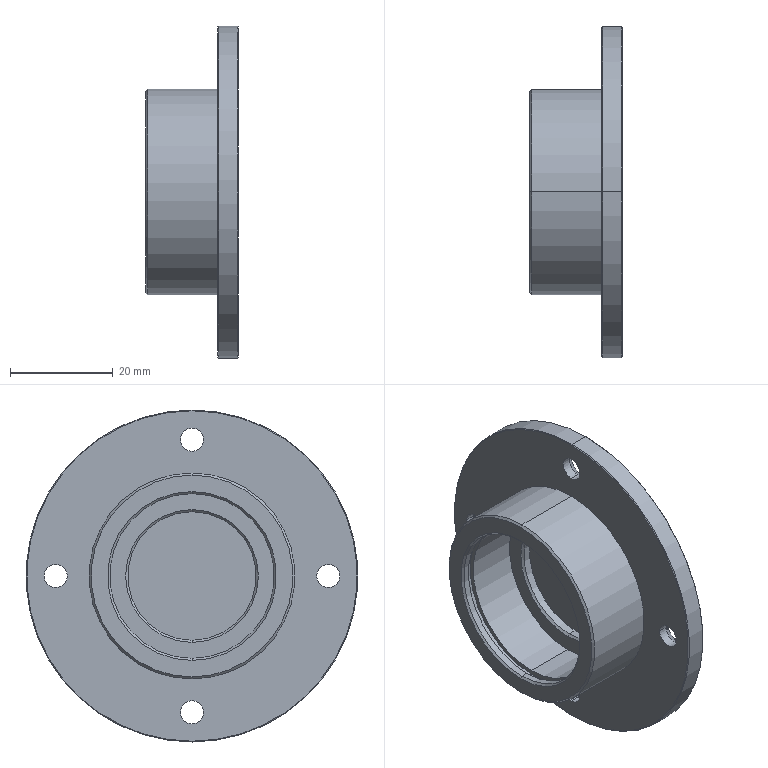Part | SolidWorks | features CirPattern 2, Chamfer 1, HoleWzd 1, ICE 1, RevCut 1, Revolution 1 | 1 solid | 45 faces | box 18 x 64.5 x 64.5 mm | volume 18637 mm3 | cylinder 20 | cone 18 | plane 7 | commonest cylinder face diameters 4.5 x8 32 x4 25 x2 33.7 x2 40 x2 64.5 x2
STEP:
#1=CARTESIAN_POINT('',(14.15,0.,32.25));
#2=VERTEX_POINT('',#1);
#3=CARTESIAN_POINT('',(14.15,0.,-32.25));
#4=VERTEX_POINT('',#3);
#5=CARTESIAN_POINT('',(14.15,0.,0.));
#6=DIRECTION('',(-1.,0.,0.));
#7=DIRECTION('',(0.,0.,-1.));
#8=AXIS2_PLACEMENT_3D('',#5,#6,#7);
#9=CIRCLE('',#8,32.25);
#10=EDGE_CURVE('',#2,#4,#9,.T.);
#11=ORIENTED_EDGE('',*,*,#10,.F.);
#12=CARTESIAN_POINT('',(17.85,0.,32.25));
#13=VERTEX_POINT('',#12);
#14=CARTESIAN_POINT('',(8.,0.,32.25));
#15=DIRECTION('',(1.,0.,0.));
#16=VECTOR('',#15,1000.);
#17=LINE('',#14,#16);
#18=EDGE_CURVE('',#2,#13,#17,.T.);
#19=ORIENTED_EDGE('',*,*,#18,.T.);
#20=CARTESIAN_POINT('',(17.85,0.,-32.25));
#21=VERTEX_POINT('',#20);
#22=CARTESIAN_POINT('',(17.85,0.,0.));
#23=DIRECTION('',(1.,0.,0.));
#24=DIRECTION('',(0.,0.,1.));
#25=AXIS2_PLACEMENT_3D('',#22,#23,#24);
#26=CIRCLE('',#25,32.25);
#27=EDGE_CURVE('',#21,#13,#26,.T.);
#28=ORIENTED_EDGE('',*,*,#27,.F.);
#29=CARTESIAN_POINT('',(8.,0.,-32.25));
#30=DIRECTION('',(1.,0.,0.));
#31=VECTOR('',#30,1000.);
#32=LINE('',#29,#31);
#33=EDGE_CURVE('',#4,#21,#32,.T.);
#34=ORIENTED_EDGE('',*,*,#33,.F.);
#35=EDGE_LOOP('',(#11,#19,#28,#34));
#36=FACE_OUTER_BOUND('',#35,.T.);
#37=CARTESIAN_POINT('',(8.,0.,0.));
#38=DIRECTION('',(1.,0.,0.));
#39=DIRECTION('',(0.,0.,-1.));
#40=AXIS2_PLACEMENT_3D('',#37,#38,#39);
#41=CYLINDRICAL_SURFACE('',#40,32.25);
#42=ADVANCED_FACE('',(#36),#41,.T.);
#43=CARTESIAN_POINT('',(0.,0.,19.6));
#44=VERTEX_POINT('',#43);
#45=CARTESIAN_POINT('',(0.,0.,-19.6));
#46=VERTEX_POINT('',#45);
#47=CARTESIAN_POINT('',(0.,0.,0.));
#48=DIRECTION('',(-1.,0.,0.));
#49=DIRECTION('',(0.,0.,-1.));
#50=AXIS2_PLACEMENT_3D('',#47,#48,#49);
#51=CIRCLE('',#50,19.6);
#52=EDGE_CURVE('',#44,#46,#51,.T.);
#53=ORIENTED_EDGE('',*,*,#52,.F.);
#54=CARTESIAN_POINT('',(0.4,0.,20.));
#55=VERTEX_POINT('',#54);
#56=CARTESIAN_POINT('',(0.,0.,19.6));
#57=DIRECTION('',(0.7071,0.,0.7071));
#58=VECTOR('',#57,1000.);
#59=LINE('',#56,#58);
#60=EDGE_CURVE('',#44,#55,#59,.T.);
#61=ORIENTED_EDGE('',*,*,#60,.T.);
#62=CARTESIAN_POINT('',(0.4,0.,-20.));
#63=VERTEX_POINT('',#62);
#64=CARTESIAN_POINT('',(0.4,0.,0.));
#65=DIRECTION('',(1.,0.,0.));
#66=DIRECTION('',(0.,0.,-1.));
#67=AXIS2_PLACEMENT_3D('',#64,#65,#66);
#68=CIRCLE('',#67,20.);
#69=EDGE_CURVE('',#63,#55,#68,.T.);
#70=ORIENTED_EDGE('',*,*,#69,.F.);
#71=CARTESIAN_POINT('',(0.,0.,-19.6));
#72=DIRECTION('',(0.7071,0.,-0.7071));
#73=VECTOR('',#72,1000.);
#74=LINE('',#71,#73);
#75=EDGE_CURVE('',#46,#63,#74,.T.);
#76=ORIENTED_EDGE('',*,*,#75,.F.);
#77=EDGE_LOOP('',(#53,#61,#70,#76));
#78=FACE_OUTER_BOUND('',#77,.T.);
#79=CARTESIAN_POINT('',(0.,0.,0.));
#80=DIRECTION('',(1.,0.,0.));
#81=DIRECTION('',(0.,0.,-1.));
#82=AXIS2_PLACEMENT_3D('',#79,#80,#81);
#83=CONICAL_SURFACE('',#82,19.6,0.7854);
#84=ADVANCED_FACE('',(#78),#83,.T.);
#85=CARTESIAN_POINT('',(0.4,0.,-16.));
#86=VERTEX_POINT('',#85);
#87=CARTESIAN_POINT('',(0.4,0.,16.));
#88=VERTEX_POINT('',#87);
#89=CARTESIAN_POINT('',(0.4,0.,0.));
#90=DIRECTION('',(-1.,0.,0.));
#91=DIRECTION('',(0.,0.,-1.));
#92=AXIS2_PLACEMENT_3D('',#89,#90,#91);
#93=CIRCLE('',#92,16.);
#94=EDGE_CURVE('',#86,#88,#93,.T.);
#95=ORIENTED_EDGE('',*,*,#94,.F.);
#96=CARTESIAN_POINT('',(0.,0.,-16.4));
#97=VERTEX_POINT('',#96);
#98=CARTESIAN_POINT('',(0.4,0.,-16.));
#99=DIRECTION('',(-0.7071,0.,-0.7071));
#100=VECTOR('',#99,1000.);
#101=LINE('',#98,#100);
#102=EDGE_CURVE('',#86,#97,#101,.T.);
#103=ORIENTED_EDGE('',*,*,#102,.T.);
#104=CARTESIAN_POINT('',(0.,0.,16.4));
#105=VERTEX_POINT('',#104);
#106=CARTESIAN_POINT('',(0.,0.,0.));
#107=DIRECTION('',(1.,0.,0.));
#108=DIRECTION('',(0.,0.,-1.));
#109=AXIS2_PLACEMENT_3D('',#106,#107,#108);
#110=CIRCLE('',#109,16.4);
#111=EDGE_CURVE('',#105,#97,#110,.T.);
#112=ORIENTED_EDGE('',*,*,#111,.F.);
#113=CARTESIAN_POINT('',(0.4,0.,16.));
#114=DIRECTION('',(-0.7071,0.,0.7071));
#115=VECTOR('',#114,1000.);
#116=LINE('',#113,#115);
#117=EDGE_CURVE('',#88,#105,#116,.T.);
#118=ORIENTED_EDGE('',*,*,#117,.F.);
#119=EDGE_LOOP('',(#95,#103,#112,#118));
#120=FACE_OUTER_BOUND('',#119,.T.);
#121=CARTESIAN_POINT('',(0.4,0.,0.));
#122=DIRECTION('',(-1.,0.,0.));
#123=DIRECTION('',(0.,0.,1.));
#124=AXIS2_PLACEMENT_3D('',#121,#122,#123);
#125=CONICAL_SURFACE('',#124,16.,0.7854);
#126=ADVANCED_FACE('',(#120),#125,.F.);
#127=CARTESIAN_POINT('',(13.4,0.,-12.5));
#128=VERTEX_POINT('',#127);
#129=CARTESIAN_POINT('',(13.4,0.,12.5));
#130=VERTEX_POINT('',#129);
#131=CARTESIAN_POINT('',(13.4,0.,0.));
#132=DIRECTION('',(-1.,0.,0.));
#133=DIRECTION('',(0.,0.,-1.));
#134=AXIS2_PLACEMENT_3D('',#131,#132,#133);
#135=CIRCLE('',#134,12.5);
#136=EDGE_CURVE('',#128,#130,#135,.T.);
#137=ORIENTED_EDGE('',*,*,#136,.F.);
#138=CARTESIAN_POINT('',(13.,0.,-12.9));
#139=VERTEX_POINT('',#138);
#140=CARTESIAN_POINT('',(13.4,0.,-12.5));
#141=DIRECTION('',(-0.7071,0.,-0.7071));
#142=VECTOR('',#141,1000.);
#143=LINE('',#140,#142);
#144=EDGE_CURVE('',#128,#139,#143,.T.);
#145=ORIENTED_EDGE('',*,*,#144,.T.);
#146=CARTESIAN_POINT('',(13.,0.,12.9));
#147=VERTEX_POINT('',#146);
#148=CARTESIAN_POINT('',(13.,0.,0.));
#149=DIRECTION('',(1.,0.,0.));
#150=DIRECTION('',(0.,0.,-1.));
#151=AXIS2_PLACEMENT_3D('',#148,#149,#150);
#152=CIRCLE('',#151,12.9);
#153=EDGE_CURVE('',#147,#139,#152,.T.);
#154=ORIENTED_EDGE('',*,*,#153,.F.);
#155=CARTESIAN_POINT('',(13.4,0.,12.5));
#156=DIRECTION('',(-0.7071,0.,0.7071));
#157=VECTOR('',#156,1000.);
#158=LINE('',#155,#157);
#159=EDGE_CURVE('',#130,#147,#158,.T.);
#160=ORIENTED_EDGE('',*,*,#159,.F.);
#161=EDGE_LOOP('',(#137,#145,#154,#160));
#162=FACE_OUTER_BOUND('',#161,.T.);
#163=CARTESIAN_POINT('',(13.4,0.,0.));
#164=DIRECTION('',(-1.,0.,0.));
#165=DIRECTION('',(0.,0.,1.));
#166=AXIS2_PLACEMENT_3D('',#163,#164,#165);
#167=CONICAL_SURFACE('',#166,12.5,0.7854);
#168=ADVANCED_FACE('',(#162),#167,.F.);
#169=CARTESIAN_POINT('',(15.75,28.75,0.));
#170=VERTEX_POINT('',#169);
#171=CARTESIAN_POINT('',(15.75,24.25,0.));
#172=VERTEX_POINT('',#171);
#173=CARTESIAN_POINT('',(15.75,26.5,0.));
#174=DIRECTION('',(-1.,0.,0.));
#175=DIRECTION('',(0.,-1.,0.));
#176=AXIS2_PLACEMENT_3D('',#173,#174,#175);
#177=CIRCLE('',#176,2.25);
#178=EDGE_CURVE('',#170,#172,#177,.T.);
#179=ORIENTED_EDGE('',*,*,#178,.F.);
#180=CARTESIAN_POINT('',(14.,28.75,0.));
#181=VERTEX_POINT('',#180);
#182=CARTESIAN_POINT('',(14.,28.75,0.));
#183=DIRECTION('',(-1.,0.,0.));
#184=VECTOR('',#183,1000.);
#185=LINE('',#182,#184);
#186=EDGE_CURVE('',#170,#181,#185,.T.);
#187=ORIENTED_EDGE('',*,*,#186,.T.);
#188=CARTESIAN_POINT('',(14.,24.25,0.));
#189=VERTEX_POINT('',#188);
#190=CARTESIAN_POINT('',(14.,26.5,0.));
#191=DIRECTION('',(-1.,0.,0.));
#192=DIRECTION('',(0.,-1.,0.));
#193=AXIS2_PLACEMENT_3D('',#190,#191,#192);
#194=CIRCLE('',#193,2.25);
#195=EDGE_CURVE('',#181,#189,#194,.T.);
#196=ORIENTED_EDGE('',*,*,#195,.T.);
#197=CARTESIAN_POINT('',(14.,24.25,0.));
#198=DIRECTION('',(-1.,0.,0.));
#199=VECTOR('',#198,1000.);
#200=LINE('',#197,#199);
#201=EDGE_CURVE('',#172,#189,#200,.T.);
#202=ORIENTED_EDGE('',*,*,#201,.F.);
#203=EDGE_LOOP('',(#179,#187,#196,#202));
#204=FACE_OUTER_BOUND('',#203,.T.);
#205=CARTESIAN_POINT('',(14.,26.5,0.));
#206=DIRECTION('',(-1.,0.,0.));
#207=DIRECTION('',(0.,-1.,0.));
#208=AXIS2_PLACEMENT_3D('',#205,#206,#207);
#209=CYLINDRICAL_SURFACE('',#208,2.25);
#210=ADVANCED_FACE('',(#204),#209,.F.);
#211=ORIENTED_EDGE('',*,*,#178,.T.);
#212=CARTESIAN_POINT('',(18.,22.,0.));
#213=VERTEX_POINT('',#212);
#214=CARTESIAN_POINT('',(18.,22.,0.));
#215=DIRECTION('',(0.7071,-0.7071,0.));
#216=VECTOR('',#215,1000.);
#217=LINE('',#214,#216);
#218=EDGE_CURVE('',#172,#213,#217,.T.);
#219=ORIENTED_EDGE('',*,*,#218,.T.);
#220=CARTESIAN_POINT('',(18.,31.,0.));
#221=VERTEX_POINT('',#220);
#222=CARTESIAN_POINT('',(18.,26.5,0.));
#223=DIRECTION('',(-1.,0.,0.));
#224=DIRECTION('',(0.,-1.,0.));
#225=AXIS2_PLACEMENT_3D('',#222,#223,#224);
#226=CIRCLE('',#225,4.5);
#227=EDGE_CURVE('',#221,#213,#226,.T.);
#228=ORIENTED_EDGE('',*,*,#227,.F.);
#229=CARTESIAN_POINT('',(18.,31.,0.));
#230=DIRECTION('',(0.7071,0.7071,0.));
#231=VECTOR('',#230,1000.);
#232=LINE('',#229,#231);
#233=EDGE_CURVE('',#170,#221,#232,.T.);
#234=ORIENTED_EDGE('',*,*,#233,.F.);
#235=EDGE_LOOP('',(#211,#219,#228,#234));
#236=FACE_OUTER_BOUND('',#235,.T.);
#237=CARTESIAN_POINT('',(18.,26.5,0.));
#238=DIRECTION('',(1.,0.,0.));
#239=DIRECTION('',(0.,1.,0.));
#240=AXIS2_PLACEMENT_3D('',#237,#238,#239);
#241=CONICAL_SURFACE('',#240,4.5,0.7854);
#242=ADVANCED_FACE('',(#236),#241,.F.);
#243=CARTESIAN_POINT('',(15.75,0.,28.75));
#244=VERTEX_POINT('',#243);
#245=CARTESIAN_POINT('',(15.75,0.,24.25));
#246=VERTEX_POINT('',#245);
#247=CARTESIAN_POINT('',(15.75,0.,26.5));
#248=DIRECTION('',(-1.,0.,0.));
#249=DIRECTION('',(0.,0.,-1.));
#250=AXIS2_PLACEMENT_3D('',#247,#248,#249);
#251=CIRCLE('',#250,2.25);
#252=EDGE_CURVE('',#244,#246,#251,.T.);
#253=ORIENTED_EDGE('',*,*,#252,.F.);
#254=CARTESIAN_POINT('',(14.,0.,28.75));
#255=VERTEX_POINT('',#254);
#256=CARTESIAN_POINT('',(14.,0.,28.75));
#257=DIRECTION('',(-1.,0.,0.));
#258=VECTOR('',#257,1000.);
#259=LINE('',#256,#258);
#260=EDGE_CURVE('',#244,#255,#259,.T.);
#261=ORIENTED_EDGE('',*,*,#260,.T.);
#262=CARTESIAN_POINT('',(14.,0.,24.25));
#263=VERTEX_POINT('',#262);
#264=CARTESIAN_POINT('',(14.,0.,26.5));
#265=DIRECTION('',(-1.,0.,0.));
#266=DIRECTION('',(0.,0.,-1.));
#267=AXIS2_PLACEMENT_3D('',#264,#265,#266);
#268=CIRCLE('',#267,2.25);
#269=EDGE_CURVE('',#255,#263,#268,.T.);
#270=ORIENTED_EDGE('',*,*,#269,.T.);
#271=CARTESIAN_POINT('',(14.,0.,24.25));
#272=DIRECTION('',(-1.,0.,0.));
#273=VECTOR('',#272,1000.);
#274=LINE('',#271,#273);
#275=EDGE_CURVE('',#246,#263,#274,.T.);
#276=ORIENTED_EDGE('',*,*,#275,.F.);
#277=EDGE_LOOP('',(#253,#261,#270,#276));
#278=FACE_OUTER_BOUND('',#277,.T.);
#279=CARTESIAN_POINT('',(14.,0.,26.5));
#280=DIRECTION('',(-1.,0.,0.));
#281=DIRECTION('',(0.,0.,-1.));
#282=AXIS2_PLACEMENT_3D('',#279,#280,#281);
#283=CYLINDRICAL_SURFACE('',#282,2.25);
#284=ADVANCED_FACE('',(#278),#283,.F.);
#285=ORIENTED_EDGE('',*,*,#252,.T.);
#286=CARTESIAN_POINT('',(18.,0.,22.));
#287=VERTEX_POINT('',#286);
#288=CARTESIAN_POINT('',(18.,0.,22.));
#289=DIRECTION('',(0.7071,0.,-0.7071));
#290=VECTOR('',#289,1000.);
#291=LINE('',#288,#290);
#292=EDGE_CURVE('',#246,#287,#291,.T.);
#293=ORIENTED_EDGE('',*,*,#292,.T.);
#294=CARTESIAN_POINT('',(18.,0.,31.));
#295=VERTEX_POINT('',#294);
#296=CARTESIAN_POINT('',(18.,0.,26.5));
#297=DIRECTION('',(-1.,0.,0.));
#298=DIRECTION('',(0.,0.,-1.));
#299=AXIS2_PLACEMENT_3D('',#296,#297,#298);
#300=CIRCLE('',#299,4.5);
#301=EDGE_CURVE('',#295,#287,#300,.T.);
#302=ORIENTED_EDGE('',*,*,#301,.F.);
#303=CARTESIAN_POINT('',(18.,0.,31.));
#304=DIRECTION('',(0.7071,0.,0.7071));
#305=VECTOR('',#304,1000.);
#306=LINE('',#303,#305);
#307=EDGE_CURVE('',#244,#295,#306,.T.);
#308=ORIENTED_EDGE('',*,*,#307,.F.);
#309=EDGE_LOOP('',(#285,#293,#302,#308));
#310=FACE_OUTER_BOUND('',#309,.T.);
#311=CARTESIAN_POINT('',(18.,0.,26.5));
#312=DIRECTION('',(1.,0.,0.));
#313=DIRECTION('',(0.,0.,1.));
#314=AXIS2_PLACEMENT_3D('',#311,#312,#313);
#315=CONICAL_SURFACE('',#314,4.5,0.7854);
#316=ADVANCED_FACE('',(#310),#315,.F.);
#317=CARTESIAN_POINT('',(15.75,-28.75,0.));
#318=VERTEX_POINT('',#317);
#319=CARTESIAN_POINT('',(15.75,-24.25,0.));
#320=VERTEX_POINT('',#319);
#321=CARTESIAN_POINT('',(15.75,-26.5,0.));
#322=DIRECTION('',(-1.,0.,0.));
#323=DIRECTION('',(0.,1.,0.));
#324=AXIS2_PLACEMENT_3D('',#321,#322,#323);
#325=CIRCLE('',#324,2.25);
#326=EDGE_CURVE('',#318,#320,#325,.T.);
#327=ORIENTED_EDGE('',*,*,#326,.F.);
#328=CARTESIAN_POINT('',(14.,-28.75,0.));
#329=VERTEX_POINT('',#328);
#330=CARTESIAN_POINT('',(14.,-28.75,0.));
#331=DIRECTION('',(-1.,0.,0.));
#332=VECTOR('',#331,1000.);
#333=LINE('',#330,#332);
#334=EDGE_CURVE('',#318,#329,#333,.T.);
#335=ORIENTED_EDGE('',*,*,#334,.T.);
#336=CARTESIAN_POINT('',(14.,-24.25,0.));
#337=VERTEX_POINT('',#336);
#338=CARTESIAN_POINT('',(14.,-26.5,0.));
#339=DIRECTION('',(-1.,0.,0.));
#340=DIRECTION('',(0.,1.,0.));
#341=AXIS2_PLACEMENT_3D('',#338,#339,#340);
#342=CIRCLE('',#341,2.25);
#343=EDGE_CURVE('',#329,#337,#342,.T.);
#344=ORIENTED_EDGE('',*,*,#343,.T.);
#345=CARTESIAN_POINT('',(14.,-24.25,0.));
#346=DIRECTION('',(-1.,0.,0.));
#347=VECTOR('',#346,1000.);
#348=LINE('',#345,#347);
#349=EDGE_CURVE('',#320,#337,#348,.T.);
#350=ORIENTED_EDGE('',*,*,#349,.F.);
#351=EDGE_LOOP('',(#327,#335,#344,#350));
#352=FACE_OUTER_BOUND('',#351,.T.);
#353=CARTESIAN_POINT('',(14.,-26.5,0.));
#354=DIRECTION('',(-1.,0.,0.));
#355=DIRECTION('',(0.,1.,0.));
#356=AXIS2_PLACEMENT_3D('',#353,#354,#355);
#357=CYLINDRICAL_SURFACE('',#356,2.25);
#358=ADVANCED_FACE('',(#352),#357,.F.);
#359=ORIENTED_EDGE('',*,*,#326,.T.);
#360=CARTESIAN_POINT('',(18.,-22.,0.));
#361=VERTEX_POINT('',#360);
#362=CARTESIAN_POINT('',(18.,-22.,0.));
#363=DIRECTION('',(0.7071,0.7071,0.));
#364=VECTOR('',#363,1000.);
#365=LINE('',#362,#364);
#366=EDGE_CURVE('',#320,#361,#365,.T.);
#367=ORIENTED_EDGE('',*,*,#366,.T.);
#368=CARTESIAN_POINT('',(18.,-31.,0.));
#369=VERTEX_POINT('',#368);
#370=CARTESIAN_POINT('',(18.,-26.5,0.));
#371=DIRECTION('',(-1.,0.,0.));
#372=DIRECTION('',(0.,1.,0.));
#373=AXIS2_PLACEMENT_3D('',#370,#371,#372);
#374=CIRCLE('',#373,4.5);
#375=EDGE_CURVE('',#369,#361,#374,.T.);
#376=ORIENTED_EDGE('',*,*,#375,.F.);
#377=CARTESIAN_POINT('',(18.,-31.,0.));
#378=DIRECTION('',(0.7071,-0.7071,0.));
#379=VECTOR('',#378,1000.);
#380=LINE('',#377,#379);
#381=EDGE_CURVE('',#318,#369,#380,.T.);
#382=ORIENTED_EDGE('',*,*,#381,.F.);
#383=EDGE_LOOP('',(#359,#367,#376,#382));
#384=FACE_OUTER_BOUND('',#383,.T.);
#385=CARTESIAN_POINT('',(18.,-26.5,0.));
#386=DIRECTION('',(1.,0.,0.));
#387=DIRECTION('',(0.,-1.,0.));
#388=AXIS2_PLACEMENT_3D('',#385,#386,#387);
#389=CONICAL_SURFACE('',#388,4.5,0.7854);
#390=ADVANCED_FACE('',(#384),#389,.F.);
#391=CARTESIAN_POINT('',(15.75,0.,-28.75));
#392=VERTEX_POINT('',#391);
#393=CARTESIAN_POINT('',(15.75,0.,-24.25));
#394=VERTEX_POINT('',#393);
#395=CARTESIAN_POINT('',(15.75,0.,-26.5));
#396=DIRECTION('',(-1.,0.,0.));
#397=DIRECTION('',(0.,0.,1.));
#398=AXIS2_PLACEMENT_3D('',#395,#396,#397);
#399=CIRCLE('',#398,2.25);
#400=EDGE_CURVE('',#392,#394,#399,.T.);
#401=ORIENTED_EDGE('',*,*,#400,.F.);
#402=CARTESIAN_POINT('',(14.,0.,-28.75));
#403=VERTEX_POINT('',#402);
#404=CARTESIAN_POINT('',(14.,0.,-28.75));
#405=DIRECTION('',(-1.,0.,0.));
#406=VECTOR('',#405,1000.);
#407=LINE('',#404,#406);
#408=EDGE_CURVE('',#392,#403,#407,.T.);
#409=ORIENTED_EDGE('',*,*,#408,.T.);
#410=CARTESIAN_POINT('',(14.,0.,-24.25));
#411=VERTEX_POINT('',#410);
#412=CARTESIAN_POINT('',(14.,0.,-26.5));
#413=DIRECTION('',(-1.,0.,0.));
#414=DIRECTION('',(0.,0.,1.));
#415=AXIS2_PLACEMENT_3D('',#412,#413,#414);
#416=CIRCLE('',#415,2.25);
#417=EDGE_CURVE('',#403,#411,#416,.T.);
#418=ORIENTED_EDGE('',*,*,#417,.T.);
#419=CARTESIAN_POINT('',(14.,0.,-24.25));
#420=DIRECTION('',(-1.,0.,0.));
#421=VECTOR('',#420,1000.);
#422=LINE('',#419,#421);
#423=EDGE_CURVE('',#394,#411,#422,.T.);
#424=ORIENTED_EDGE('',*,*,#423,.F.);
#425=EDGE_LOOP('',(#401,#409,#418,#424));
#426=FACE_OUTER_BOUND('',#425,.T.);
#427=CARTESIAN_POINT('',(14.,0.,-26.5));
#428=DIRECTION('',(-1.,0.,0.));
#429=DIRECTION('',(0.,0.,1.));
#430=AXIS2_PLACEMENT_3D('',#427,#428,#429);
#431=CYLINDRICAL_SURFACE('',#430,2.25);
#432=ADVANCED_FACE('',(#426),#431,.F.);
#433=ORIENTED_EDGE('',*,*,#400,.T.);
#434=CARTESIAN_POINT('',(18.,0.,-22.));
#435=VERTEX_POINT('',#434);
#436=CARTESIAN_POINT('',(18.,0.,-22.));
#437=DIRECTION('',(0.7071,0.,0.7071));
#438=VECTOR('',#437,1000.);
#439=LINE('',#436,#438);
#440=EDGE_CURVE('',#394,#435,#439,.T.);
#441=ORIENTED_EDGE('',*,*,#440,.T.);
#442=CARTESIAN_POINT('',(18.,0.,-31.));
#443=VERTEX_POINT('',#442);
#444=CARTESIAN_POINT('',(18.,0.,-26.5));
#445=DIRECTION('',(-1.,0.,0.));
#446=DIRECTION('',(0.,0.,1.));
#447=AXIS2_PLACEMENT_3D('',#444,#445,#446);
#448=CIRCLE('',#447,4.5);
#449=EDGE_CURVE('',#443,#435,#448,.T.);
#450=ORIENTED_EDGE('',*,*,#449,.F.);
#451=CARTESIAN_POINT('',(18.,0.,-31.));
#452=DIRECTION('',(0.7071,0.,-0.7071));
#453=VECTOR('',#452,1000.);
#454=LINE('',#451,#453);
#455=EDGE_CURVE('',#392,#443,#454,.T.);
#456=ORIENTED_EDGE('',*,*,#455,.F.);
#457=EDGE_LOOP('',(#433,#441,#450,#456));
#458=FACE_OUTER_BOUND('',#457,.T.);
#459=CARTESIAN_POINT('',(18.,0.,-26.5));
#460=DIRECTION('',(1.,0.,0.));
#461=DIRECTION('',(0.,0.,-1.));
#462=AXIS2_PLACEMENT_3D('',#459,#460,#461);
#463=CONICAL_SURFACE('',#462,4.5,0.7854);
#464=ADVANCED_FACE('',(#458),#463,.F.);
#465=CARTESIAN_POINT('',(14.,0.,20.));
#466=VERTEX_POINT('',#465);
#467=CARTESIAN_POINT('',(14.,0.,-20.));
#468=VERTEX_POINT('',#467);
#469=CARTESIAN_POINT('',(14.,0.,0.));
#470=DIRECTION('',(-1.,0.,0.));
#471=DIRECTION('',(0.,0.,1.));
#472=AXIS2_PLACEMENT_3D('',#469,#470,#471);
#473=CIRCLE('',#472,20.);
#474=EDGE_CURVE('',#466,#468,#473,.T.);
#475=ORIENTED_EDGE('',*,*,#474,.T.);
#476=CARTESIAN_POINT('',(15.,0.,-20.));
#477=DIRECTION('',(-1.,0.,0.));
#478=VECTOR('',#477,1000.);
#479=LINE('',#476,#478);
#480=EDGE_CURVE('',#468,#63,#479,.T.);
#481=ORIENTED_EDGE('',*,*,#480,.T.);
#482=ORIENTED_EDGE('',*,*,#69,.T.);
#483=CARTESIAN_POINT('',(15.,0.,20.));
#484=DIRECTION('',(-1.,0.,0.));
#485=VECTOR('',#484,1000.);
#486=LINE('',#483,#485);
#487=EDGE_CURVE('',#466,#55,#486,.T.);
#488=ORIENTED_EDGE('',*,*,#487,.F.);
#489=EDGE_LOOP('',(#475,#481,#482,#488));
#490=FACE_OUTER_BOUND('',#489,.T.);
#491=CARTESIAN_POINT('',(15.,0.,0.));
#492=DIRECTION('',(-1.,0.,0.));
#493=DIRECTION('',(0.,0.,1.));
#494=AXIS2_PLACEMENT_3D('',#491,#492,#493);
#495=CYLINDRICAL_SURFACE('',#494,20.);
#496=ADVANCED_FACE('',(#490),#495,.T.);
#497=CARTESIAN_POINT('',(15.,0.,-12.5));
#498=VERTEX_POINT('',#497);
#499=CARTESIAN_POINT('',(15.,0.,12.5));
#500=VERTEX_POINT('',#499);
#501=CARTESIAN_POINT('',(15.,0.,0.));
#502=DIRECTION('',(-1.,0.,0.));
#503=DIRECTION('',(0.,0.,1.));
#504=AXIS2_PLACEMENT_3D('',#501,#502,#503);
#505=CIRCLE('',#504,12.5);
#506=EDGE_CURVE('',#498,#500,#505,.T.);
#507=ORIENTED_EDGE('',*,*,#506,.F.);
#508=CARTESIAN_POINT('',(15.,0.,-12.5));
#509=DIRECTION('',(-1.,0.,0.));
#510=VECTOR('',#509,1000.);
#511=LINE('',#508,#510);
#512=EDGE_CURVE('',#498,#128,#511,.T.);
#513=ORIENTED_EDGE('',*,*,#512,.T.);
#514=ORIENTED_EDGE('',*,*,#136,.T.);
#515=CARTESIAN_POINT('',(15.,0.,12.5));
#516=DIRECTION('',(-1.,0.,0.));
#517=VECTOR('',#516,1000.);
#518=LINE('',#515,#517);
#519=EDGE_CURVE('',#500,#130,#518,.T.);
#520=ORIENTED_EDGE('',*,*,#519,.F.);
#521=EDGE_LOOP('',(#507,#513,#514,#520));
#522=FACE_OUTER_BOUND('',#521,.T.);
#523=CARTESIAN_POINT('',(15.,0.,0.));
#524=DIRECTION('',(-1.,0.,0.));
#525=DIRECTION('',(0.,0.,1.));
#526=AXIS2_PLACEMENT_3D('',#523,#524,#525);
#527=CYLINDRICAL_SURFACE('',#526,12.5);
#528=ADVANCED_FACE('',(#522),#527,.F.);
#529=CARTESIAN_POINT('',(13.,0.,-16.));
#530=VERTEX_POINT('',#529);
#531=CARTESIAN_POINT('',(13.,0.,16.));
#532=VERTEX_POINT('',#531);
#533=CARTESIAN_POINT('',(13.,0.,0.));
#534=DIRECTION('',(-1.,0.,0.));
#535=DIRECTION('',(0.,0.,1.));
#536=AXIS2_PLACEMENT_3D('',#533,#534,#535);
#537=CIRCLE('',#536,16.);
#538=EDGE_CURVE('',#530,#532,#537,.T.);
#539=ORIENTED_EDGE('',*,*,#538,.F.);
#540=CARTESIAN_POINT('',(2.995,0.,-16.));
#541=VERTEX_POINT('',#540);
#542=CARTESIAN_POINT('',(15.,0.,-16.));
#543=DIRECTION('',(-1.,0.,0.));
#544=VECTOR('',#543,1000.);
#545=LINE('',#542,#544);
#546=EDGE_CURVE('',#530,#541,#545,.T.);
#547=ORIENTED_EDGE('',*,*,#546,.T.);
#548=CARTESIAN_POINT('',(2.995,0.,16.));
#549=VERTEX_POINT('',#548);
#550=CARTESIAN_POINT('',(2.995,0.,0.));
#551=DIRECTION('',(-1.,0.,0.));
#552=DIRECTION('',(0.,0.,1.));
#553=AXIS2_PLACEMENT_3D('',#550,#551,#552);
#554=CIRCLE('',#553,16.);
#555=EDGE_CURVE('',#541,#549,#554,.T.);
#556=ORIENTED_EDGE('',*,*,#555,.T.);
#557=CARTESIAN_POINT('',(15.,0.,16.));
#558=DIRECTION('',(-1.,0.,0.));
#559=VECTOR('',#558,1000.);
#560=LINE('',#557,#559);
#561=EDGE_CURVE('',#532,#549,#560,.T.);
#562=ORIENTED_EDGE('',*,*,#561,.F.);
#563=EDGE_LOOP('',(#539,#547,#556,#562));
#564=FACE_OUTER_BOUND('',#563,.T.);
#565=CARTESIAN_POINT('',(15.,0.,0.));
#566=DIRECTION('',(-1.,0.,0.));
#567=DIRECTION('',(0.,0.,1.));
#568=AXIS2_PLACEMENT_3D('',#565,#566,#567);
#569=CYLINDRICAL_SURFACE('',#568,16.);
#570=ADVANCED_FACE('',(#564),#569,.F.);
#571=CARTESIAN_POINT('',(2.995,0.,-16.85));
#572=VERTEX_POINT('',#571);
#573=CARTESIAN_POINT('',(2.995,0.,16.85));
#574=VERTEX_POINT('',#573);
#575=CARTESIAN_POINT('',(2.995,0.,0.));
#576=DIRECTION('',(-1.,0.,0.));
#577=DIRECTION('',(0.,0.,1.));
#578=AXIS2_PLACEMENT_3D('',#575,#576,#577);
#579=CIRCLE('',#578,16.85);
#580=EDGE_CURVE('',#572,#574,#579,.T.);
#581=ORIENTED_EDGE('',*,*,#580,.F.);
#582=CARTESIAN_POINT('',(1.695,0.,-16.85));
#583=VERTEX_POINT('',#582);
#584=CARTESIAN_POINT('',(15.,0.,-16.85));
#585=DIRECTION('',(-1.,0.,0.));
#586=VECTOR('',#585,1000.);
#587=LINE('',#584,#586);
#588=EDGE_CURVE('',#572,#583,#587,.T.);
#589=ORIENTED_EDGE('',*,*,#588,.T.);
#590=CARTESIAN_POINT('',(1.695,0.,16.85));
#591=VERTEX_POINT('',#590);
#592=CARTESIAN_POINT('',(1.695,0.,0.));
#593=DIRECTION('',(-1.,0.,0.));
#594=DIRECTION('',(0.,0.,1.));
#595=AXIS2_PLACEMENT_3D('',#592,#593,#594);
#596=CIRCLE('',#595,16.85);
#597=EDGE_CURVE('',#583,#591,#596,.T.);
#598=ORIENTED_EDGE('',*,*,#597,.T.);
#599=CARTESIAN_POINT('',(15.,0.,16.85));
#600=DIRECTION('',(-1.,0.,0.));
#601=VECTOR('',#600,1000.);
#602=LINE('',#599,#601);
#603=EDGE_CURVE('',#574,#591,#602,.T.);
#604=ORIENTED_EDGE('',*,*,#603,.F.);
#605=EDGE_LOOP('',(#581,#589,#598,#604));
#606=FACE_OUTER_BOUND('',#605,.T.);
#607=CARTESIAN_POINT('',(15.,0.,0.));
#608=DIRECTION('',(-1.,0.,0.));
#609=DIRECTION('',(0.,0.,1.));
#610=AXIS2_PLACEMENT_3D('',#607,#608,#609);
#611=CYLINDRICAL_SURFACE('',#610,16.85);
#612=ADVANCED_FACE('',(#606),#611,.F.);
#613=CARTESIAN_POINT('',(1.695,0.,-16.));
#614=VERTEX_POINT('',#613);
#615=CARTESIAN_POINT('',(1.695,0.,16.));
#616=VERTEX_POINT('',#615);
#617=CARTESIAN_POINT('',(1.695,0.,0.));
#618=DIRECTION('',(-1.,0.,0.));
#619=DIRECTION('',(0.,0.,1.));
#620=AXIS2_PLACEMENT_3D('',#617,#618,#619);
#621=CIRCLE('',#620,16.);
#622=EDGE_CURVE('',#614,#616,#621,.T.);
#623=ORIENTED_EDGE('',*,*,#622,.F.);
#624=CARTESIAN_POINT('',(15.,0.,-16.));
#625=DIRECTION('',(-1.,0.,0.));
#626=VECTOR('',#625,1000.);
#627=LINE('',#624,#626);
#628=EDGE_CURVE('',#614,#86,#627,.T.);
#629=ORIENTED_EDGE('',*,*,#628,.T.);
#630=ORIENTED_EDGE('',*,*,#94,.T.);
#631=CARTESIAN_POINT('',(15.,0.,16.));
#632=DIRECTION('',(-1.,0.,0.));
#633=VECTOR('',#632,1000.);
#634=LINE('',#631,#633);
#635=EDGE_CURVE('',#616,#88,#634,.T.);
#636=ORIENTED_EDGE('',*,*,#635,.F.);
#637=EDGE_LOOP('',(#623,#629,#630,#636));
#638=FACE_OUTER_BOUND('',#637,.T.);
#639=CARTESIAN_POINT('',(15.,0.,0.));
#640=DIRECTION('',(-1.,0.,0.));
#641=DIRECTION('',(0.,0.,1.));
#642=AXIS2_PLACEMENT_3D('',#639,#640,#641);
#643=CYLINDRICAL_SURFACE('',#642,16.);
#644=ADVANCED_FACE('',(#638),#643,.F.);
#645=CARTESIAN_POINT('',(14.,0.,32.1));
#646=VERTEX_POINT('',#645);
#647=CARTESIAN_POINT('',(14.,0.,-32.1));
#648=VERTEX_POINT('',#647);
#649=CARTESIAN_POINT('',(14.,0.,0.));
#650=DIRECTION('',(-1.,0.,0.));
#651=DIRECTION('',(0.,0.,-1.));
#652=AXIS2_PLACEMENT_3D('',#649,#650,#651);
#653=CIRCLE('',#652,32.1);
#654=EDGE_CURVE('',#646,#648,#653,.T.);
#655=ORIENTED_EDGE('',*,*,#654,.F.);
#656=CARTESIAN_POINT('',(14.,0.,32.1));
#657=DIRECTION('',(0.7071,0.,0.7071));
#658=VECTOR('',#657,1000.);
#659=LINE('',#656,#658);
#660=EDGE_CURVE('',#646,#2,#659,.T.);
#661=ORIENTED_EDGE('',*,*,#660,.T.);
#662=ORIENTED_EDGE('',*,*,#10,.T.);
#663=CARTESIAN_POINT('',(14.,0.,-32.1));
#664=DIRECTION('',(0.7071,0.,-0.7071));
#665=VECTOR('',#664,1000.);
#666=LINE('',#663,#665);
#667=EDGE_CURVE('',#648,#4,#666,.T.);
#668=ORIENTED_EDGE('',*,*,#667,.F.);
#669=EDGE_LOOP('',(#655,#661,#662,#668));
#670=FACE_OUTER_BOUND('',#669,.T.);
#671=CARTESIAN_POINT('',(14.,0.,0.));
#672=DIRECTION('',(1.,0.,0.));
#673=DIRECTION('',(0.,0.,-1.));
#674=AXIS2_PLACEMENT_3D('',#671,#672,#673);
#675=CONICAL_SURFACE('',#674,32.1,0.7854);
#676=ADVANCED_FACE('',(#670),#675,.T.);
#677=CARTESIAN_POINT('',(18.,0.,-32.1));
#678=VERTEX_POINT('',#677);
#679=CARTESIAN_POINT('',(18.,0.,32.1));
#680=VERTEX_POINT('',#679);
#681=CARTESIAN_POINT('',(18.,0.,0.));
#682=DIRECTION('',(1.,0.,0.));
#683=DIRECTION('',(0.,0.,1.));
#684=AXIS2_PLACEMENT_3D('',#681,#682,#683);
#685=CIRCLE('',#684,32.1);
#686=EDGE_CURVE('',#678,#680,#685,.T.);
#687=ORIENTED_EDGE('',*,*,#686,.F.);
#688=CARTESIAN_POINT('',(17.6,0.,-32.5));
#689=DIRECTION('',(-0.7071,0.,-0.7071));
#690=VECTOR('',#689,1000.);
#691=LINE('',#688,#690);
#692=EDGE_CURVE('',#678,#21,#691,.T.);
#693=ORIENTED_EDGE('',*,*,#692,.T.);
#694=ORIENTED_EDGE('',*,*,#27,.T.);
#695=CARTESIAN_POINT('',(17.6,0.,32.5));
#696=DIRECTION('',(-0.7071,0.,0.7071));
#697=VECTOR('',#696,1000.);
#698=LINE('',#695,#697);
#699=EDGE_CURVE('',#680,#13,#698,.T.);
#700=ORIENTED_EDGE('',*,*,#699,.F.);
#701=EDGE_LOOP('',(#687,#693,#694,#700));
#702=FACE_OUTER_BOUND('',#701,.T.);
#703=CARTESIAN_POINT('',(17.6,0.,0.));
#704=DIRECTION('',(-1.,0.,0.));
#705=DIRECTION('',(0.,0.,1.));
#706=AXIS2_PLACEMENT_3D('',#703,#704,#705);
#707=CONICAL_SURFACE('',#706,32.5,0.7854);
#708=ADVANCED_FACE('',(#702),#707,.T.);
#709=ORIENTED_EDGE('',*,*,#692,.F.);
#710=CARTESIAN_POINT('',(18.,0.,0.));
#711=DIRECTION('',(1.,0.,0.));
#712=DIRECTION('',(0.,0.,1.));
#713=AXIS2_PLACEMENT_3D('',#710,#711,#712);
#714=CIRCLE('',#713,32.1);
#715=EDGE_CURVE('',#680,#678,#714,.T.);
#716=ORIENTED_EDGE('',*,*,#715,.F.);
#717=ORIENTED_EDGE('',*,*,#699,.T.);
#718=CARTESIAN_POINT('',(17.85,0.,0.));
#719=DIRECTION('',(1.,0.,0.));
#720=DIRECTION('',(0.,0.,1.));
#721=AXIS2_PLACEMENT_3D('',#718,#719,#720);
#722=CIRCLE('',#721,32.25);
#723=EDGE_CURVE('',#13,#21,#722,.T.);
#724=ORIENTED_EDGE('',*,*,#723,.T.);
#725=EDGE_LOOP('',(#709,#716,#717,#724));
#726=FACE_OUTER_BOUND('',#725,.T.);
#727=CARTESIAN_POINT('',(17.6,0.,0.));
#728=DIRECTION('',(-1.,0.,0.));
#729=DIRECTION('',(0.,0.,1.));
#730=AXIS2_PLACEMENT_3D('',#727,#728,#729);
#731=CONICAL_SURFACE('',#730,32.5,0.7854);
#732=ADVANCED_FACE('',(#726),#731,.T.);
#733=ORIENTED_EDGE('',*,*,#660,.F.);
#734=CARTESIAN_POINT('',(14.,0.,0.));
#735=DIRECTION('',(-1.,0.,0.));
#736=DIRECTION('',(0.,0.,-1.));
#737=AXIS2_PLACEMENT_3D('',#734,#735,#736);
#738=CIRCLE('',#737,32.1);
#739=EDGE_CURVE('',#648,#646,#738,.T.);
#740=ORIENTED_EDGE('',*,*,#739,.F.);
#741=ORIENTED_EDGE('',*,*,#667,.T.);
#742=CARTESIAN_POINT('',(14.15,0.,0.));
#743=DIRECTION('',(-1.,0.,0.));
#744=DIRECTION('',(0.,0.,-1.));
#745=AXIS2_PLACEMENT_3D('',#742,#743,#744);
#746=CIRCLE('',#745,32.25);
#747=EDGE_CURVE('',#4,#2,#746,.T.);
#748=ORIENTED_EDGE('',*,*,#747,.T.);
#749=EDGE_LOOP('',(#733,#740,#741,#748));
#750=FACE_OUTER_BOUND('',#749,.T.);
#751=CARTESIAN_POINT('',(14.,0.,0.));
#752=DIRECTION('',(1.,0.,0.));
#753=DIRECTION('',(0.,0.,-1.));
#754=AXIS2_PLACEMENT_3D('',#751,#752,#753);
#755=CONICAL_SURFACE('',#754,32.1,0.7854);
#756=ADVANCED_FACE('',(#750),#755,.T.);
#757=ORIENTED_EDGE('',*,*,#111,.T.);
#758=CARTESIAN_POINT('',(0.,0.,0.));
#759=DIRECTION('',(1.,0.,0.));
#760=DIRECTION('',(0.,0.,-1.));
#761=AXIS2_PLACEMENT_3D('',#758,#759,#760);
#762=CIRCLE('',#761,16.4);
#763=EDGE_CURVE('',#97,#105,#762,.T.);
#764=ORIENTED_EDGE('',*,*,#763,.T.);
#765=EDGE_LOOP('',(#757,#764));
#766=FACE_BOUND('',#765,.T.);
#767=CARTESIAN_POINT('',(0.,0.,0.));
#768=DIRECTION('',(-1.,0.,0.));
#769=DIRECTION('',(0.,0.,-1.));
#770=AXIS2_PLACEMENT_3D('',#767,#768,#769);
#771=CIRCLE('',#770,19.6);
#772=EDGE_CURVE('',#46,#44,#771,.T.);
#773=ORIENTED_EDGE('',*,*,#772,.T.);
#774=ORIENTED_EDGE('',*,*,#52,.T.);
#775=EDGE_LOOP('',(#773,#774));
#776=FACE_OUTER_BOUND('',#775,.T.);
#777=CARTESIAN_POINT('',(0.,20.,0.));
#778=DIRECTION('',(1.,0.,0.));
#779=DIRECTION('',(0.,0.,-1.));
#780=AXIS2_PLACEMENT_3D('',#777,#778,#779);
#781=PLANE('',#780);
#782=ADVANCED_FACE('',(#766,#776),#781,.F.);
#783=ORIENTED_EDGE('',*,*,#628,.F.);
#784=CARTESIAN_POINT('',(1.695,0.,0.));
#785=DIRECTION('',(-1.,0.,0.));
#786=DIRECTION('',(0.,0.,1.));
#787=AXIS2_PLACEMENT_3D('',#784,#785,#786);
#788=CIRCLE('',#787,16.);
#789=EDGE_CURVE('',#616,#614,#788,.T.);
#790=ORIENTED_EDGE('',*,*,#789,.F.);
#791=ORIENTED_EDGE('',*,*,#635,.T.);
#792=CARTESIAN_POINT('',(0.4,0.,0.));
#793=DIRECTION('',(-1.,0.,0.));
#794=DIRECTION('',(0.,0.,-1.));
#795=AXIS2_PLACEMENT_3D('',#792,#793,#794);
#796=CIRCLE('',#795,16.);
#797=EDGE_CURVE('',#88,#86,#796,.T.);
#798=ORIENTED_EDGE('',*,*,#797,.T.);
#799=EDGE_LOOP('',(#783,#790,#791,#798));
#800=FACE_OUTER_BOUND('',#799,.T.);
#801=CARTESIAN_POINT('',(15.,0.,0.));
#802=DIRECTION('',(-1.,0.,0.));
#803=DIRECTION('',(0.,0.,1.));
#804=AXIS2_PLACEMENT_3D('',#801,#802,#803);
#805=CYLINDRICAL_SURFACE('',#804,16.);
#806=ADVANCED_FACE('',(#800),#805,.F.);
#807=CARTESIAN_POINT('',(1.695,0.,0.));
#808=DIRECTION('',(-1.,0.,0.));
#809=DIRECTION('',(0.,0.,1.));
#810=AXIS2_PLACEMENT_3D('',#807,#808,#809);
#811=CIRCLE('',#810,16.85);
#812=EDGE_CURVE('',#591,#583,#811,.T.);
#813=ORIENTED_EDGE('',*,*,#812,.F.);
#814=ORIENTED_EDGE('',*,*,#597,.F.);
#815=EDGE_LOOP('',(#813,#814));
#816=FACE_OUTER_BOUND('',#815,.T.);
#817=ORIENTED_EDGE('',*,*,#789,.T.);
#818=ORIENTED_EDGE('',*,*,#622,.T.);
#819=EDGE_LOOP('',(#817,#818));
#820=FACE_BOUND('',#819,.T.);
#821=CARTESIAN_POINT('',(1.695,16.,0.));
#822=DIRECTION('',(-1.,0.,0.));
#823=DIRECTION('',(0.,0.,1.));
#824=AXIS2_PLACEMENT_3D('',#821,#822,#823);
#825=PLANE('',#824);
#826=ADVANCED_FACE('',(#816,#820),#825,.F.);
#827=ORIENTED_EDGE('',*,*,#588,.F.);
#828=CARTESIAN_POINT('',(2.995,0.,0.));
#829=DIRECTION('',(-1.,0.,0.));
#830=DIRECTION('',(0.,0.,1.));
#831=AXIS2_PLACEMENT_3D('',#828,#829,#830);
#832=CIRCLE('',#831,16.85);
#833=EDGE_CURVE('',#574,#572,#832,.T.);
#834=ORIENTED_EDGE('',*,*,#833,.F.);
#835=ORIENTED_EDGE('',*,*,#603,.T.);
#836=ORIENTED_EDGE('',*,*,#812,.T.);
#837=EDGE_LOOP('',(#827,#834,#835,#836));
#838=FACE_OUTER_BOUND('',#837,.T.);
#839=CARTESIAN_POINT('',(15.,0.,0.));
#840=DIRECTION('',(-1.,0.,0.));
#841=DIRECTION('',(0.,0.,1.));
#842=AXIS2_PLACEMENT_3D('',#839,#840,#841);
#843=CYLINDRICAL_SURFACE('',#842,16.85);
#844=ADVANCED_FACE('',(#838),#843,.F.);
#845=CARTESIAN_POINT('',(2.995,0.,0.));
#846=DIRECTION('',(-1.,0.,0.));
#847=DIRECTION('',(0.,0.,1.));
#848=AXIS2_PLACEMENT_3D('',#845,#846,#847);
#849=CIRCLE('',#848,16.);
#850=EDGE_CURVE('',#549,#541,#849,.T.);
#851=ORIENTED_EDGE('',*,*,#850,.F.);
#852=ORIENTED_EDGE('',*,*,#555,.F.);
#853=EDGE_LOOP('',(#851,#852));
#854=FACE_BOUND('',#853,.T.);
#855=ORIENTED_EDGE('',*,*,#833,.T.);
#856=ORIENTED_EDGE('',*,*,#580,.T.);
#857=EDGE_LOOP('',(#855,#856));
#858=FACE_OUTER_BOUND('',#857,.T.);
#859=CARTESIAN_POINT('',(2.995,16.85,0.));
#860=DIRECTION('',(1.,0.,0.));
#861=DIRECTION('',(0.,0.,-1.));
#862=AXIS2_PLACEMENT_3D('',#859,#860,#861);
#863=PLANE('',#862);
#864=ADVANCED_FACE('',(#854,#858),#863,.F.);
#865=ORIENTED_EDGE('',*,*,#546,.F.);
#866=CARTESIAN_POINT('',(13.,0.,0.));
#867=DIRECTION('',(-1.,0.,0.));
#868=DIRECTION('',(0.,0.,1.));
#869=AXIS2_PLACEMENT_3D('',#866,#867,#868);
#870=CIRCLE('',#869,16.);
#871=EDGE_CURVE('',#532,#530,#870,.T.);
#872=ORIENTED_EDGE('',*,*,#871,.F.);
#873=ORIENTED_EDGE('',*,*,#561,.T.);
#874=ORIENTED_EDGE('',*,*,#850,.T.);
#875=EDGE_LOOP('',(#865,#872,#873,#874));
#876=FACE_OUTER_BOUND('',#875,.T.);
#877=CARTESIAN_POINT('',(15.,0.,0.));
#878=DIRECTION('',(-1.,0.,0.));
#879=DIRECTION('',(0.,0.,1.));
#880=AXIS2_PLACEMENT_3D('',#877,#878,#879);
#881=CYLINDRICAL_SURFACE('',#880,16.);
#882=ADVANCED_FACE('',(#876),#881,.F.);
#883=ORIENTED_EDGE('',*,*,#153,.T.);
#884=CARTESIAN_POINT('',(13.,0.,0.));
#885=DIRECTION('',(1.,0.,0.));
#886=DIRECTION('',(0.,0.,-1.));
#887=AXIS2_PLACEMENT_3D('',#884,#885,#886);
#888=CIRCLE('',#887,12.9);
#889=EDGE_CURVE('',#139,#147,#888,.T.);
#890=ORIENTED_EDGE('',*,*,#889,.T.);
#891=EDGE_LOOP('',(#883,#890));
#892=FACE_BOUND('',#891,.T.);
#893=ORIENTED_EDGE('',*,*,#871,.T.);
#894=ORIENTED_EDGE('',*,*,#538,.T.);
#895=EDGE_LOOP('',(#893,#894));
#896=FACE_OUTER_BOUND('',#895,.T.);
#897=CARTESIAN_POINT('',(13.,16.,0.));
#898=DIRECTION('',(1.,0.,0.));
#899=DIRECTION('',(0.,0.,-1.));
#900=AXIS2_PLACEMENT_3D('',#897,#898,#899);
#901=PLANE('',#900);
#902=ADVANCED_FACE('',(#892,#896),#901,.F.);
#903=ORIENTED_EDGE('',*,*,#512,.F.);
#904=CARTESIAN_POINT('',(15.,0.,0.));
#905=DIRECTION('',(-1.,0.,0.));
#906=DIRECTION('',(0.,0.,1.));
#907=AXIS2_PLACEMENT_3D('',#904,#905,#906);
#908=CIRCLE('',#907,12.5);
#909=EDGE_CURVE('',#500,#498,#908,.T.);
#910=ORIENTED_EDGE('',*,*,#909,.F.);
#911=ORIENTED_EDGE('',*,*,#519,.T.);
#912=CARTESIAN_POINT('',(13.4,0.,0.));
#913=DIRECTION('',(-1.,0.,0.));
#914=DIRECTION('',(0.,0.,-1.));
#915=AXIS2_PLACEMENT_3D('',#912,#913,#914);
#916=CIRCLE('',#915,12.5);
#917=EDGE_CURVE('',#130,#128,#916,.T.);
#918=ORIENTED_EDGE('',*,*,#917,.T.);
#919=EDGE_LOOP('',(#903,#910,#911,#918));
#920=FACE_OUTER_BOUND('',#919,.T.);
#921=CARTESIAN_POINT('',(15.,0.,0.));
#922=DIRECTION('',(-1.,0.,0.));
#923=DIRECTION('',(0.,0.,1.));
#924=AXIS2_PLACEMENT_3D('',#921,#922,#923);
#925=CYLINDRICAL_SURFACE('',#924,12.5);
#926=ADVANCED_FACE('',(#920),#925,.F.);
#927=ORIENTED_EDGE('',*,*,#909,.T.);
#928=ORIENTED_EDGE('',*,*,#506,.T.);
#929=EDGE_LOOP('',(#927,#928));
#930=FACE_OUTER_BOUND('',#929,.T.);
#931=CARTESIAN_POINT('',(15.,12.5,0.));
#932=DIRECTION('',(1.,0.,0.));
#933=DIRECTION('',(0.,0.,-1.));
#934=AXIS2_PLACEMENT_3D('',#931,#932,#933);
#935=PLANE('',#934);
#936=ADVANCED_FACE('',(#930),#935,.F.);
#937=ORIENTED_EDGE('',*,*,#715,.T.);
#938=ORIENTED_EDGE('',*,*,#686,.T.);
#939=EDGE_LOOP('',(#937,#938));
#940=FACE_OUTER_BOUND('',#939,.T.);
#941=ORIENTED_EDGE('',*,*,#227,.T.);
#942=CARTESIAN_POINT('',(18.,26.5,0.));
#943=DIRECTION('',(-1.,0.,0.));
#944=DIRECTION('',(0.,-1.,0.));
#945=AXIS2_PLACEMENT_3D('',#942,#943,#944);
#946=CIRCLE('',#945,4.5);
#947=EDGE_CURVE('',#213,#221,#946,.T.);
#948=ORIENTED_EDGE('',*,*,#947,.T.);
#949=EDGE_LOOP('',(#941,#948));
#950=FACE_BOUND('',#949,.T.);
#951=ORIENTED_EDGE('',*,*,#301,.T.);
#952=CARTESIAN_POINT('',(18.,0.,26.5));
#953=DIRECTION('',(-1.,0.,0.));
#954=DIRECTION('',(0.,0.,-1.));
#955=AXIS2_PLACEMENT_3D('',#952,#953,#954);
#956=CIRCLE('',#955,4.5);
#957=EDGE_CURVE('',#287,#295,#956,.T.);
#958=ORIENTED_EDGE('',*,*,#957,.T.);
#959=EDGE_LOOP('',(#951,#958));
#960=FACE_BOUND('',#959,.T.);
#961=ORIENTED_EDGE('',*,*,#375,.T.);
#962=CARTESIAN_POINT('',(18.,-26.5,0.));
#963=DIRECTION('',(-1.,0.,0.));
#964=DIRECTION('',(0.,1.,0.));
#965=AXIS2_PLACEMENT_3D('',#962,#963,#964);
#966=CIRCLE('',#965,4.5);
#967=EDGE_CURVE('',#361,#369,#966,.T.);
#968=ORIENTED_EDGE('',*,*,#967,.T.);
#969=EDGE_LOOP('',(#961,#968));
#970=FACE_BOUND('',#969,.T.);
#971=ORIENTED_EDGE('',*,*,#449,.T.);
#972=CARTESIAN_POINT('',(18.,0.,-26.5));
#973=DIRECTION('',(-1.,0.,0.));
#974=DIRECTION('',(0.,0.,1.));
#975=AXIS2_PLACEMENT_3D('',#972,#973,#974);
#976=CIRCLE('',#975,4.5);
#977=EDGE_CURVE('',#435,#443,#976,.T.);
#978=ORIENTED_EDGE('',*,*,#977,.T.);
#979=EDGE_LOOP('',(#971,#978));
#980=FACE_BOUND('',#979,.T.);
#981=CARTESIAN_POINT('',(18.,0.,0.));
#982=DIRECTION('',(-1.,0.,0.));
#983=DIRECTION('',(0.,0.,1.));
#984=AXIS2_PLACEMENT_3D('',#981,#982,#983);
#985=PLANE('',#984);
#986=ADVANCED_FACE('',(#940,#950,#960,#970,#980),#985,.F.);
#987=ORIENTED_EDGE('',*,*,#739,.T.);
#988=ORIENTED_EDGE('',*,*,#654,.T.);
#989=EDGE_LOOP('',(#987,#988));
#990=FACE_OUTER_BOUND('',#989,.T.);
#991=CARTESIAN_POINT('',(14.,26.5,0.));
#992=DIRECTION('',(-1.,0.,0.));
#993=DIRECTION('',(0.,-1.,0.));
#994=AXIS2_PLACEMENT_3D('',#991,#992,#993);
#995=CIRCLE('',#994,2.25);
#996=EDGE_CURVE('',#189,#181,#995,.T.);
#997=ORIENTED_EDGE('',*,*,#996,.F.);
#998=ORIENTED_EDGE('',*,*,#195,.F.);
#999=EDGE_LOOP('',(#997,#998));
#1000=FACE_BOUND('',#999,.T.);
#1001=CARTESIAN_POINT('',(14.,0.,26.5));
#1002=DIRECTION('',(-1.,0.,0.));
#1003=DIRECTION('',(0.,0.,-1.));
#1004=AXIS2_PLACEMENT_3D('',#1001,#1002,#1003);
#1005=CIRCLE('',#1004,2.25);
#1006=EDGE_CURVE('',#263,#255,#1005,.T.);
#1007=ORIENTED_EDGE('',*,*,#1006,.F.);
#1008=ORIENTED_EDGE('',*,*,#269,.F.);
#1009=EDGE_LOOP('',(#1007,#1008));
#1010=FACE_BOUND('',#1009,.T.);
#1011=CARTESIAN_POINT('',(14.,-26.5,0.));
#1012=DIRECTION('',(-1.,0.,0.));
#1013=DIRECTION('',(0.,1.,0.));
#1014=AXIS2_PLACEMENT_3D('',#1011,#1012,#1013);
#1015=CIRCLE('',#1014,2.25);
#1016=EDGE_CURVE('',#337,#329,#1015,.T.);
#1017=ORIENTED_EDGE('',*,*,#1016,.F.);
#1018=ORIENTED_EDGE('',*,*,#343,.F.);
#1019=EDGE_LOOP('',(#1017,#1018));
#1020=FACE_BOUND('',#1019,.T.);
#1021=CARTESIAN_POINT('',(14.,0.,-26.5));
#1022=DIRECTION('',(-1.,0.,0.));
#1023=DIRECTION('',(0.,0.,1.));
#1024=AXIS2_PLACEMENT_3D('',#1021,#1022,#1023);
#1025=CIRCLE('',#1024,2.25);
#1026=EDGE_CURVE('',#411,#403,#1025,.T.);
#1027=ORIENTED_EDGE('',*,*,#1026,.F.);
#1028=ORIENTED_EDGE('',*,*,#417,.F.);
#1029=EDGE_LOOP('',(#1027,#1028));
#1030=FACE_BOUND('',#1029,.T.);
#1031=ORIENTED_EDGE('',*,*,#474,.F.);
#1032=CARTESIAN_POINT('',(14.,0.,0.));
#1033=DIRECTION('',(-1.,0.,0.));
#1034=DIRECTION('',(0.,0.,1.));
#1035=AXIS2_PLACEMENT_3D('',#1032,#1033,#1034);
#1036=CIRCLE('',#1035,20.);
#1037=EDGE_CURVE('',#468,#466,#1036,.T.);
#1038=ORIENTED_EDGE('',*,*,#1037,.F.);
#1039=EDGE_LOOP('',(#1031,#1038));
#1040=FACE_BOUND('',#1039,.T.);
#1041=CARTESIAN_POINT('',(14.,32.5,0.));
#1042=DIRECTION('',(1.,0.,0.));
#1043=DIRECTION('',(0.,0.,-1.));
#1044=AXIS2_PLACEMENT_3D('',#1041,#1042,#1043);
#1045=PLANE('',#1044);
#1046=ADVANCED_FACE('',(#990,#1000,#1010,#1020,#1030,#1040),#1045,.F.);
#1047=ORIENTED_EDGE('',*,*,#480,.F.);
#1048=ORIENTED_EDGE('',*,*,#1037,.T.);
#1049=ORIENTED_EDGE('',*,*,#487,.T.);
#1050=CARTESIAN_POINT('',(0.4,0.,0.));
#1051=DIRECTION('',(1.,0.,0.));
#1052=DIRECTION('',(0.,0.,-1.));
#1053=AXIS2_PLACEMENT_3D('',#1050,#1051,#1052);
#1054=CIRCLE('',#1053,20.);
#1055=EDGE_CURVE('',#55,#63,#1054,.T.);
#1056=ORIENTED_EDGE('',*,*,#1055,.T.);
#1057=EDGE_LOOP('',(#1047,#1048,#1049,#1056));
#1058=FACE_OUTER_BOUND('',#1057,.T.);
#1059=CARTESIAN_POINT('',(15.,0.,0.));
#1060=DIRECTION('',(-1.,0.,0.));
#1061=DIRECTION('',(0.,0.,1.));
#1062=AXIS2_PLACEMENT_3D('',#1059,#1060,#1061);
#1063=CYLINDRICAL_SURFACE('',#1062,20.);
#1064=ADVANCED_FACE('',(#1058),#1063,.T.);
#1065=ORIENTED_EDGE('',*,*,#440,.F.);
#1066=CARTESIAN_POINT('',(15.75,0.,-26.5));
#1067=DIRECTION('',(-1.,0.,0.));
#1068=DIRECTION('',(0.,0.,1.));
#1069=AXIS2_PLACEMENT_3D('',#1066,#1067,#1068);
#1070=CIRCLE('',#1069,2.25);
#1071=EDGE_CURVE('',#394,#392,#1070,.T.);
#1072=ORIENTED_EDGE('',*,*,#1071,.T.);
#1073=ORIENTED_EDGE('',*,*,#455,.T.);
#1074=ORIENTED_EDGE('',*,*,#977,.F.);
#1075=EDGE_LOOP('',(#1065,#1072,#1073,#1074));
#1076=FACE_OUTER_BOUND('',#1075,.T.);
#1077=CARTESIAN_POINT('',(18.,0.,-26.5));
#1078=DIRECTION('',(1.,0.,0.));
#1079=DIRECTION('',(0.,0.,-1.));
#1080=AXIS2_PLACEMENT_3D('',#1077,#1078,#1079);
#1081=CONICAL_SURFACE('',#1080,4.5,0.7854);
#1082=ADVANCED_FACE('',(#1076),#1081,.F.);
#1083=ORIENTED_EDGE('',*,*,#408,.F.);
#1084=ORIENTED_EDGE('',*,*,#1071,.F.);
#1085=ORIENTED_EDGE('',*,*,#423,.T.);
#1086=ORIENTED_EDGE('',*,*,#1026,.T.);
#1087=EDGE_LOOP('',(#1083,#1084,#1085,#1086));
#1088=FACE_OUTER_BOUND('',#1087,.T.);
#1089=CARTESIAN_POINT('',(14.,0.,-26.5));
#1090=DIRECTION('',(-1.,0.,0.));
#1091=DIRECTION('',(0.,0.,1.));
#1092=AXIS2_PLACEMENT_3D('',#1089,#1090,#1091);
#1093=CYLINDRICAL_SURFACE('',#1092,2.25);
#1094=ADVANCED_FACE('',(#1088),#1093,.F.);
#1095=ORIENTED_EDGE('',*,*,#366,.F.);
#1096=CARTESIAN_POINT('',(15.75,-26.5,0.));
#1097=DIRECTION('',(-1.,0.,0.));
#1098=DIRECTION('',(0.,1.,0.));
#1099=AXIS2_PLACEMENT_3D('',#1096,#1097,#1098);
#1100=CIRCLE('',#1099,2.25);
#1101=EDGE_CURVE('',#320,#318,#1100,.T.);
#1102=ORIENTED_EDGE('',*,*,#1101,.T.);
#1103=ORIENTED_EDGE('',*,*,#381,.T.);
#1104=ORIENTED_EDGE('',*,*,#967,.F.);
#1105=EDGE_LOOP('',(#1095,#1102,#1103,#1104));
#1106=FACE_OUTER_BOUND('',#1105,.T.);
#1107=CARTESIAN_POINT('',(18.,-26.5,0.));
#1108=DIRECTION('',(1.,0.,0.));
#1109=DIRECTION('',(0.,-1.,0.));
#1110=AXIS2_PLACEMENT_3D('',#1107,#1108,#1109);
#1111=CONICAL_SURFACE('',#1110,4.5,0.7854);
#1112=ADVANCED_FACE('',(#1106),#1111,.F.);
#1113=ORIENTED_EDGE('',*,*,#334,.F.);
#1114=ORIENTED_EDGE('',*,*,#1101,.F.);
#1115=ORIENTED_EDGE('',*,*,#349,.T.);
#1116=ORIENTED_EDGE('',*,*,#1016,.T.);
#1117=EDGE_LOOP('',(#1113,#1114,#1115,#1116));
#1118=FACE_OUTER_BOUND('',#1117,.T.);
#1119=CARTESIAN_POINT('',(14.,-26.5,0.));
#1120=DIRECTION('',(-1.,0.,0.));
#1121=DIRECTION('',(0.,1.,0.));
#1122=AXIS2_PLACEMENT_3D('',#1119,#1120,#1121);
#1123=CYLINDRICAL_SURFACE('',#1122,2.25);
#1124=ADVANCED_FACE('',(#1118),#1123,.F.);
#1125=ORIENTED_EDGE('',*,*,#292,.F.);
#1126=CARTESIAN_POINT('',(15.75,0.,26.5));
#1127=DIRECTION('',(-1.,0.,0.));
#1128=DIRECTION('',(0.,0.,-1.));
#1129=AXIS2_PLACEMENT_3D('',#1126,#1127,#1128);
#1130=CIRCLE('',#1129,2.25);
#1131=EDGE_CURVE('',#246,#244,#1130,.T.);
#1132=ORIENTED_EDGE('',*,*,#1131,.T.);
#1133=ORIENTED_EDGE('',*,*,#307,.T.);
#1134=ORIENTED_EDGE('',*,*,#957,.F.);
#1135=EDGE_LOOP('',(#1125,#1132,#1133,#1134));
#1136=FACE_OUTER_BOUND('',#1135,.T.);
#1137=CARTESIAN_POINT('',(18.,0.,26.5));
#1138=DIRECTION('',(1.,0.,0.));
#1139=DIRECTION('',(0.,0.,1.));
#1140=AXIS2_PLACEMENT_3D('',#1137,#1138,#1139);
#1141=CONICAL_SURFACE('',#1140,4.5,0.7854);
#1142=ADVANCED_FACE('',(#1136),#1141,.F.);
#1143=ORIENTED_EDGE('',*,*,#260,.F.);
#1144=ORIENTED_EDGE('',*,*,#1131,.F.);
#1145=ORIENTED_EDGE('',*,*,#275,.T.);
#1146=ORIENTED_EDGE('',*,*,#1006,.T.);
#1147=EDGE_LOOP('',(#1143,#1144,#1145,#1146));
#1148=FACE_OUTER_BOUND('',#1147,.T.);
#1149=CARTESIAN_POINT('',(14.,0.,26.5));
#1150=DIRECTION('',(-1.,0.,0.));
#1151=DIRECTION('',(0.,0.,-1.));
#1152=AXIS2_PLACEMENT_3D('',#1149,#1150,#1151);
#1153=CYLINDRICAL_SURFACE('',#1152,2.25);
#1154=ADVANCED_FACE('',(#1148),#1153,.F.);
#1155=ORIENTED_EDGE('',*,*,#218,.F.);
#1156=CARTESIAN_POINT('',(15.75,26.5,0.));
#1157=DIRECTION('',(-1.,0.,0.));
#1158=DIRECTION('',(0.,-1.,0.));
#1159=AXIS2_PLACEMENT_3D('',#1156,#1157,#1158);
#1160=CIRCLE('',#1159,2.25);
#1161=EDGE_CURVE('',#172,#170,#1160,.T.);
#1162=ORIENTED_EDGE('',*,*,#1161,.T.);
#1163=ORIENTED_EDGE('',*,*,#233,.T.);
#1164=ORIENTED_EDGE('',*,*,#947,.F.);
#1165=EDGE_LOOP('',(#1155,#1162,#1163,#1164));
#1166=FACE_OUTER_BOUND('',#1165,.T.);
#1167=CARTESIAN_POINT('',(18.,26.5,0.));
#1168=DIRECTION('',(1.,0.,0.));
#1169=DIRECTION('',(0.,1.,0.));
#1170=AXIS2_PLACEMENT_3D('',#1167,#1168,#1169);
#1171=CONICAL_SURFACE('',#1170,4.5,0.7854);
#1172=ADVANCED_FACE('',(#1166),#1171,.F.);
#1173=ORIENTED_EDGE('',*,*,#186,.F.);
#1174=ORIENTED_EDGE('',*,*,#1161,.F.);
#1175=ORIENTED_EDGE('',*,*,#201,.T.);
#1176=ORIENTED_EDGE('',*,*,#996,.T.);
#1177=EDGE_LOOP('',(#1173,#1174,#1175,#1176));
#1178=FACE_OUTER_BOUND('',#1177,.T.);
#1179=CARTESIAN_POINT('',(14.,26.5,0.));
#1180=DIRECTION('',(-1.,0.,0.));
#1181=DIRECTION('',(0.,-1.,0.));
#1182=AXIS2_PLACEMENT_3D('',#1179,#1180,#1181);
#1183=CYLINDRICAL_SURFACE('',#1182,2.25);
#1184=ADVANCED_FACE('',(#1178),#1183,.F.);
#1185=ORIENTED_EDGE('',*,*,#144,.F.);
#1186=ORIENTED_EDGE('',*,*,#917,.F.);
#1187=ORIENTED_EDGE('',*,*,#159,.T.);
#1188=ORIENTED_EDGE('',*,*,#889,.F.);
#1189=EDGE_LOOP('',(#1185,#1186,#1187,#1188));
#1190=FACE_OUTER_BOUND('',#1189,.T.);
#1191=CARTESIAN_POINT('',(13.4,0.,0.));
#1192=DIRECTION('',(-1.,0.,0.));
#1193=DIRECTION('',(0.,0.,1.));
#1194=AXIS2_PLACEMENT_3D('',#1191,#1192,#1193);
#1195=CONICAL_SURFACE('',#1194,12.5,0.7854);
#1196=ADVANCED_FACE('',(#1190),#1195,.F.);
#1197=ORIENTED_EDGE('',*,*,#102,.F.);
#1198=ORIENTED_EDGE('',*,*,#797,.F.);
#1199=ORIENTED_EDGE('',*,*,#117,.T.);
#1200=ORIENTED_EDGE('',*,*,#763,.F.);
#1201=EDGE_LOOP('',(#1197,#1198,#1199,#1200));
#1202=FACE_OUTER_BOUND('',#1201,.T.);
#1203=CARTESIAN_POINT('',(0.4,0.,0.));
#1204=DIRECTION('',(-1.,0.,0.));
#1205=DIRECTION('',(0.,0.,1.));
#1206=AXIS2_PLACEMENT_3D('',#1203,#1204,#1205);
#1207=CONICAL_SURFACE('',#1206,16.,0.7854);
#1208=ADVANCED_FACE('',(#1202),#1207,.F.);
#1209=ORIENTED_EDGE('',*,*,#60,.F.);
#1210=ORIENTED_EDGE('',*,*,#772,.F.);
#1211=ORIENTED_EDGE('',*,*,#75,.T.);
#1212=ORIENTED_EDGE('',*,*,#1055,.F.);
#1213=EDGE_LOOP('',(#1209,#1210,#1211,#1212));
#1214=FACE_OUTER_BOUND('',#1213,.T.);
#1215=CARTESIAN_POINT('',(0.,0.,0.));
#1216=DIRECTION('',(1.,0.,0.));
#1217=DIRECTION('',(0.,0.,-1.));
#1218=AXIS2_PLACEMENT_3D('',#1215,#1216,#1217);
#1219=CONICAL_SURFACE('',#1218,19.6,0.7854);
#1220=ADVANCED_FACE('',(#1214),#1219,.T.);
#1221=ORIENTED_EDGE('',*,*,#18,.F.);
#1222=ORIENTED_EDGE('',*,*,#747,.F.);
#1223=ORIENTED_EDGE('',*,*,#33,.T.);
#1224=ORIENTED_EDGE('',*,*,#723,.F.);
#1225=EDGE_LOOP('',(#1221,#1222,#1223,#1224));
#1226=FACE_OUTER_BOUND('',#1225,.T.);
#1227=CARTESIAN_POINT('',(8.,0.,0.));
#1228=DIRECTION('',(1.,0.,0.));
#1229=DIRECTION('',(0.,0.,-1.));
#1230=AXIS2_PLACEMENT_3D('',#1227,#1228,#1229);
#1231=CYLINDRICAL_SURFACE('',#1230,32.25);
#1232=ADVANCED_FACE('',(#1226),#1231,.T.);
#1233=CLOSED_SHELL('',(#42,#84,#126,#168,#210,#242,#284,#316,#358,#390,#432,#464,#496,#528,#570,#612,#644,#676,#708,#732,#756,#782,#806,#826,#844,#864,#882,#902,#926,#936,#986,#1046,#1064,#1082,#1094,#1112,#1124,#1142,#1154,#1172,#1184,#1196,#1208,#1220,#1232));
#1234=MANIFOLD_SOLID_BREP('',#1233);
#1235=CARTESIAN_POINT('',(0.,0.,0.));
#1236=DIRECTION('',(0.,0.,1.));
#1237=DIRECTION('',(1.,0.,0.));
#1238=AXIS2_PLACEMENT_3D('',#1235,#1236,#1237);
#1239=(LENGTH_UNIT()NAMED_UNIT(*)SI_UNIT(.MILLI.,.METRE.));
#1240=UNCERTAINTY_MEASURE_WITH_UNIT(LENGTH_MEASURE(0.00001),#1239,'','');
#1241=(NAMED_UNIT(*)PLANE_ANGLE_UNIT()SI_UNIT($,.RADIAN.));
#1242=(NAMED_UNIT(*)SI_UNIT($,.STERADIAN.)SOLID_ANGLE_UNIT());
#1243=(GEOMETRIC_REPRESENTATION_CONTEXT(3)GLOBAL_UNCERTAINTY_ASSIGNED_CONTEXT((#1240))GLOBAL_UNIT_ASSIGNED_CONTEXT((#1239,#1241,#1242))REPRESENTATION_CONTEXT('',''));
#1244=ADVANCED_BREP_SHAPE_REPRESENTATION('',(#1234,#1238),#1243);